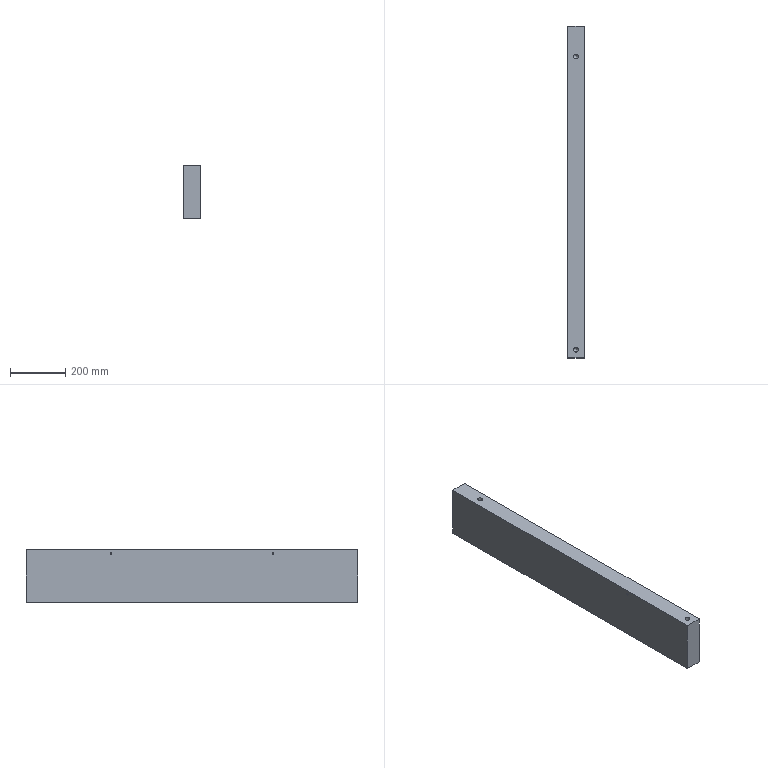Part | STEP file | lll_id4634_x_t | 1 solid | 34 faces | box 60 x 1200 x 190 mm | volume 13627617 mm3 | cylinder 14 | cone 14 | plane 6 | commonest cylinder face diameters 6.806 x10 17.506 x4
STEP:
#1=CARTESIAN_POINT('',(3946.188,490.,-370.));
#2=VERTEX_POINT('',#1);
#3=CARTESIAN_POINT('',(3937.435,490.,-370.));
#4=DIRECTION('',(0.,0.,1.));
#5=DIRECTION('',(1.,0.,0.));
#6=AXIS2_PLACEMENT_3D('',#3,#4,#5);
#7=CIRCLE('',#6,8.753);
#8=EDGE_CURVE('',#2,#2,#7,.T.);
#9=ORIENTED_EDGE('',*,*,#8,.T.);
#10=EDGE_LOOP('',(#9));
#11=FACE_BOUND('',#10,.T.);
#12=CARTESIAN_POINT('',(3907.435,-600.,-370.));
#13=VERTEX_POINT('',#12);
#14=CARTESIAN_POINT('',(3967.435,-600.,-370.));
#15=VERTEX_POINT('',#14);
#16=CARTESIAN_POINT('',(6153.751,-600.,-370.));
#17=DIRECTION('',(1.,0.,0.));
#18=VECTOR('',#17,1.);
#19=LINE('',#16,#18);
#20=EDGE_CURVE('',#13,#15,#19,.T.);
#21=ORIENTED_EDGE('',*,*,#20,.F.);
#22=CARTESIAN_POINT('',(3907.435,600.,-370.));
#23=VERTEX_POINT('',#22);
#24=CARTESIAN_POINT('',(3907.435,-1.,-370.));
#25=DIRECTION('',(0.,1.,0.));
#26=VECTOR('',#25,1.);
#27=LINE('',#24,#26);
#28=EDGE_CURVE('',#13,#23,#27,.T.);
#29=ORIENTED_EDGE('',*,*,#28,.T.);
#30=CARTESIAN_POINT('',(3967.435,600.,-370.));
#31=VERTEX_POINT('',#30);
#32=CARTESIAN_POINT('',(3967.435,600.,-370.));
#33=DIRECTION('',(-1.,0.,0.));
#34=VECTOR('',#33,1.);
#35=LINE('',#32,#34);
#36=EDGE_CURVE('',#31,#23,#35,.T.);
#37=ORIENTED_EDGE('',*,*,#36,.F.);
#38=CARTESIAN_POINT('',(3967.435,-600.,-370.));
#39=DIRECTION('',(0.,1.,0.));
#40=VECTOR('',#39,1.);
#41=LINE('',#38,#40);
#42=EDGE_CURVE('',#15,#31,#41,.T.);
#43=ORIENTED_EDGE('',*,*,#42,.F.);
#44=EDGE_LOOP('',(#21,#29,#37,#43));
#45=FACE_BOUND('',#44,.T.);
#46=CARTESIAN_POINT('',(3946.188,-490.,-370.));
#47=VERTEX_POINT('',#46);
#48=CARTESIAN_POINT('',(3937.435,-490.,-370.));
#49=DIRECTION('',(0.,0.,1.));
#50=DIRECTION('',(1.,0.,0.));
#51=AXIS2_PLACEMENT_3D('',#48,#49,#50);
#52=CIRCLE('',#51,8.753);
#53=EDGE_CURVE('',#47,#47,#52,.T.);
#54=ORIENTED_EDGE('',*,*,#53,.T.);
#55=EDGE_LOOP('',(#54));
#56=FACE_BOUND('',#55,.T.);
#57=CARTESIAN_POINT('',(6153.751,-1.,-370.));
#58=DIRECTION('',(0.,0.,-1.));
#59=DIRECTION('',(-1.,0.,0.));
#60=AXIS2_PLACEMENT_3D('',#57,#58,#59);
#61=PLANE('',#60);
#62=ADVANCED_FACE('',(#11,#45,#56),#61,.T.);
#63=CARTESIAN_POINT('',(3907.435,600.,-180.));
#64=VERTEX_POINT('',#63);
#65=CARTESIAN_POINT('',(3907.435,600.,-182.5));
#66=DIRECTION('',(0.,0.,-1.));
#67=VECTOR('',#66,1.);
#68=LINE('',#65,#67);
#69=EDGE_CURVE('',#64,#23,#68,.T.);
#70=ORIENTED_EDGE('',*,*,#69,.F.);
#71=CARTESIAN_POINT('',(3967.435,600.,-180.));
#72=VERTEX_POINT('',#71);
#73=CARTESIAN_POINT('',(6153.751,600.,-180.));
#74=DIRECTION('',(-1.,0.,0.));
#75=VECTOR('',#74,1.);
#76=LINE('',#73,#75);
#77=EDGE_CURVE('',#72,#64,#76,.T.);
#78=ORIENTED_EDGE('',*,*,#77,.F.);
#79=CARTESIAN_POINT('',(3967.435,600.,-182.5));
#80=DIRECTION('',(0.,0.,-1.));
#81=VECTOR('',#80,1.);
#82=LINE('',#79,#81);
#83=EDGE_CURVE('',#72,#31,#82,.T.);
#84=ORIENTED_EDGE('',*,*,#83,.T.);
#85=ORIENTED_EDGE('',*,*,#36,.T.);
#86=EDGE_LOOP('',(#70,#78,#84,#85));
#87=FACE_OUTER_BOUND('',#86,.T.);
#88=CARTESIAN_POINT('',(3967.435,600.,-182.5));
#89=DIRECTION('',(0.,1.,0.));
#90=DIRECTION('',(0.,0.,-1.));
#91=AXIS2_PLACEMENT_3D('',#88,#89,#90);
#92=PLANE('',#91);
#93=ADVANCED_FACE('',(#87),#92,.T.);
#94=CARTESIAN_POINT('',(3907.435,-289.597,-194.165));
#95=VERTEX_POINT('',#94);
#96=CARTESIAN_POINT('',(3907.435,-293.,-194.165));
#97=DIRECTION('',(1.,0.,0.));
#98=DIRECTION('',(0.,1.,0.));
#99=AXIS2_PLACEMENT_3D('',#96,#97,#98);
#100=CIRCLE('',#99,3.403);
#101=EDGE_CURVE('',#95,#95,#100,.T.);
#102=ORIENTED_EDGE('',*,*,#101,.T.);
#103=EDGE_LOOP('',(#102));
#104=FACE_BOUND('',#103,.T.);
#105=CARTESIAN_POINT('',(3907.435,296.403,-194.165));
#106=VERTEX_POINT('',#105);
#107=CARTESIAN_POINT('',(3907.435,293.,-194.165));
#108=DIRECTION('',(1.,0.,0.));
#109=DIRECTION('',(0.,1.,0.));
#110=AXIS2_PLACEMENT_3D('',#107,#108,#109);
#111=CIRCLE('',#110,3.403);
#112=EDGE_CURVE('',#106,#106,#111,.T.);
#113=ORIENTED_EDGE('',*,*,#112,.T.);
#114=EDGE_LOOP('',(#113));
#115=FACE_BOUND('',#114,.T.);
#116=CARTESIAN_POINT('',(3907.435,-600.,-180.));
#117=VERTEX_POINT('',#116);
#118=CARTESIAN_POINT('',(3907.435,0.,-180.));
#119=DIRECTION('',(0.,-1.,0.));
#120=VECTOR('',#119,1.);
#121=LINE('',#118,#120);
#122=EDGE_CURVE('',#64,#117,#121,.T.);
#123=ORIENTED_EDGE('',*,*,#122,.F.);
#124=ORIENTED_EDGE('',*,*,#69,.T.);
#125=ORIENTED_EDGE('',*,*,#28,.F.);
#126=CARTESIAN_POINT('',(3907.435,-600.,-160.));
#127=DIRECTION('',(0.,0.,-1.));
#128=VECTOR('',#127,1.);
#129=LINE('',#126,#128);
#130=EDGE_CURVE('',#117,#13,#129,.T.);
#131=ORIENTED_EDGE('',*,*,#130,.F.);
#132=EDGE_LOOP('',(#123,#124,#125,#131));
#133=FACE_BOUND('',#132,.T.);
#134=CARTESIAN_POINT('',(3907.435,0.,-251.25));
#135=DIRECTION('',(1.,0.,0.));
#136=DIRECTION('',(0.,0.,-1.));
#137=AXIS2_PLACEMENT_3D('',#134,#135,#136);
#138=PLANE('',#137);
#139=ADVANCED_FACE('',(#104,#115,#133),#138,.F.);
#140=CARTESIAN_POINT('',(3928.682,490.,-180.));
#141=VERTEX_POINT('',#140);
#142=CARTESIAN_POINT('',(3937.435,490.,-180.));
#143=DIRECTION('',(0.,0.,-1.));
#144=DIRECTION('',(-1.,0.,0.));
#145=AXIS2_PLACEMENT_3D('',#142,#143,#144);
#146=CIRCLE('',#145,8.753);
#147=EDGE_CURVE('',#141,#141,#146,.T.);
#148=ORIENTED_EDGE('',*,*,#147,.T.);
#149=EDGE_LOOP('',(#148));
#150=FACE_BOUND('',#149,.T.);
#151=CARTESIAN_POINT('',(3928.682,-570.,-180.));
#152=VERTEX_POINT('',#151);
#153=CARTESIAN_POINT('',(3937.435,-570.,-180.));
#154=DIRECTION('',(0.,0.,-1.));
#155=DIRECTION('',(-1.,0.,0.));
#156=AXIS2_PLACEMENT_3D('',#153,#154,#155);
#157=CIRCLE('',#156,8.753);
#158=EDGE_CURVE('',#152,#152,#157,.T.);
#159=ORIENTED_EDGE('',*,*,#158,.T.);
#160=EDGE_LOOP('',(#159));
#161=FACE_BOUND('',#160,.T.);
#162=CARTESIAN_POINT('',(3967.435,-600.,-180.));
#163=VERTEX_POINT('',#162);
#164=CARTESIAN_POINT('',(3967.435,-1.,-180.));
#165=DIRECTION('',(0.,1.,0.));
#166=VECTOR('',#165,1.);
#167=LINE('',#164,#166);
#168=EDGE_CURVE('',#163,#72,#167,.T.);
#169=ORIENTED_EDGE('',*,*,#168,.T.);
#170=ORIENTED_EDGE('',*,*,#77,.T.);
#171=ORIENTED_EDGE('',*,*,#122,.T.);
#172=CARTESIAN_POINT('',(2132.435,-600.,-180.));
#173=DIRECTION('',(-1.,0.,0.));
#174=VECTOR('',#173,1.);
#175=LINE('',#172,#174);
#176=EDGE_CURVE('',#163,#117,#175,.T.);
#177=ORIENTED_EDGE('',*,*,#176,.F.);
#178=EDGE_LOOP('',(#169,#170,#171,#177));
#179=FACE_BOUND('',#178,.T.);
#180=CARTESIAN_POINT('',(6153.751,-1.,-180.));
#181=DIRECTION('',(0.,0.,-1.));
#182=DIRECTION('',(-1.,0.,0.));
#183=AXIS2_PLACEMENT_3D('',#180,#181,#182);
#184=PLANE('',#183);
#185=ADVANCED_FACE('',(#150,#161,#179),#184,.F.);
#186=CARTESIAN_POINT('',(3967.435,402.5,-254.597));
#187=VERTEX_POINT('',#186);
#188=CARTESIAN_POINT('',(3967.435,402.5,-258.));
#189=DIRECTION('',(-1.,0.,0.));
#190=DIRECTION('',(0.,0.,1.));
#191=AXIS2_PLACEMENT_3D('',#188,#189,#190);
#192=CIRCLE('',#191,3.403);
#193=EDGE_CURVE('',#187,#187,#192,.T.);
#194=ORIENTED_EDGE('',*,*,#193,.T.);
#195=EDGE_LOOP('',(#194));
#196=FACE_BOUND('',#195,.T.);
#197=CARTESIAN_POINT('',(3967.435,412.5,-224.597));
#198=VERTEX_POINT('',#197);
#199=CARTESIAN_POINT('',(3967.435,412.5,-228.));
#200=DIRECTION('',(-1.,0.,0.));
#201=DIRECTION('',(0.,0.,1.));
#202=AXIS2_PLACEMENT_3D('',#199,#200,#201);
#203=CIRCLE('',#202,3.403);
#204=EDGE_CURVE('',#198,#198,#203,.T.);
#205=ORIENTED_EDGE('',*,*,#204,.T.);
#206=EDGE_LOOP('',(#205));
#207=FACE_BOUND('',#206,.T.);
#208=CARTESIAN_POINT('',(3967.435,62.5,-254.597));
#209=VERTEX_POINT('',#208);
#210=CARTESIAN_POINT('',(3967.435,62.5,-258.));
#211=DIRECTION('',(-1.,0.,0.));
#212=DIRECTION('',(0.,0.,1.));
#213=AXIS2_PLACEMENT_3D('',#210,#211,#212);
#214=CIRCLE('',#213,3.403);
#215=EDGE_CURVE('',#209,#209,#214,.T.);
#216=ORIENTED_EDGE('',*,*,#215,.T.);
#217=EDGE_LOOP('',(#216));
#218=FACE_BOUND('',#217,.T.);
#219=CARTESIAN_POINT('',(3967.435,72.5,-224.597));
#220=VERTEX_POINT('',#219);
#221=CARTESIAN_POINT('',(3967.435,72.5,-228.));
#222=DIRECTION('',(-1.,0.,0.));
#223=DIRECTION('',(0.,0.,1.));
#224=AXIS2_PLACEMENT_3D('',#221,#222,#223);
#225=CIRCLE('',#224,3.403);
#226=EDGE_CURVE('',#220,#220,#225,.T.);
#227=ORIENTED_EDGE('',*,*,#226,.T.);
#228=EDGE_LOOP('',(#227));
#229=FACE_BOUND('',#228,.T.);
#230=CARTESIAN_POINT('',(3967.435,-82.,-254.597));
#231=VERTEX_POINT('',#230);
#232=CARTESIAN_POINT('',(3967.435,-82.,-258.));
#233=DIRECTION('',(-1.,0.,0.));
#234=DIRECTION('',(0.,0.,1.));
#235=AXIS2_PLACEMENT_3D('',#232,#233,#234);
#236=CIRCLE('',#235,3.403);
#237=EDGE_CURVE('',#231,#231,#236,.T.);
#238=ORIENTED_EDGE('',*,*,#237,.T.);
#239=EDGE_LOOP('',(#238));
#240=FACE_BOUND('',#239,.T.);
#241=CARTESIAN_POINT('',(3967.435,-72.,-224.597));
#242=VERTEX_POINT('',#241);
#243=CARTESIAN_POINT('',(3967.435,-72.,-228.));
#244=DIRECTION('',(-1.,0.,0.));
#245=DIRECTION('',(0.,0.,1.));
#246=AXIS2_PLACEMENT_3D('',#243,#244,#245);
#247=CIRCLE('',#246,3.403);
#248=EDGE_CURVE('',#242,#242,#247,.T.);
#249=ORIENTED_EDGE('',*,*,#248,.T.);
#250=EDGE_LOOP('',(#249));
#251=FACE_BOUND('',#250,.T.);
#252=CARTESIAN_POINT('',(3967.435,-422.,-254.597));
#253=VERTEX_POINT('',#252);
#254=CARTESIAN_POINT('',(3967.435,-422.,-258.));
#255=DIRECTION('',(-1.,0.,0.));
#256=DIRECTION('',(0.,0.,1.));
#257=AXIS2_PLACEMENT_3D('',#254,#255,#256);
#258=CIRCLE('',#257,3.403);
#259=EDGE_CURVE('',#253,#253,#258,.T.);
#260=ORIENTED_EDGE('',*,*,#259,.T.);
#261=EDGE_LOOP('',(#260));
#262=FACE_BOUND('',#261,.T.);
#263=CARTESIAN_POINT('',(3967.435,-412.,-224.597));
#264=VERTEX_POINT('',#263);
#265=CARTESIAN_POINT('',(3967.435,-412.,-228.));
#266=DIRECTION('',(-1.,0.,0.));
#267=DIRECTION('',(0.,0.,1.));
#268=AXIS2_PLACEMENT_3D('',#265,#266,#267);
#269=CIRCLE('',#268,3.403);
#270=EDGE_CURVE('',#264,#264,#269,.T.);
#271=ORIENTED_EDGE('',*,*,#270,.T.);
#272=EDGE_LOOP('',(#271));
#273=FACE_BOUND('',#272,.T.);
#274=CARTESIAN_POINT('',(3967.435,-600.,-160.));
#275=DIRECTION('',(0.,0.,-1.));
#276=VECTOR('',#275,1.);
#277=LINE('',#274,#276);
#278=EDGE_CURVE('',#163,#15,#277,.T.);
#279=ORIENTED_EDGE('',*,*,#278,.T.);
#280=ORIENTED_EDGE('',*,*,#42,.T.);
#281=ORIENTED_EDGE('',*,*,#83,.F.);
#282=ORIENTED_EDGE('',*,*,#168,.F.);
#283=EDGE_LOOP('',(#279,#280,#281,#282));
#284=FACE_BOUND('',#283,.T.);
#285=CARTESIAN_POINT('',(3967.435,-600.,-182.5));
#286=DIRECTION('',(1.,0.,0.));
#287=DIRECTION('',(0.,0.,-1.));
#288=AXIS2_PLACEMENT_3D('',#285,#286,#287);
#289=PLANE('',#288);
#290=ADVANCED_FACE('',(#196,#207,#218,#229,#240,#251,#262,#273,#284),#289,.T.);
#291=ORIENTED_EDGE('',*,*,#278,.F.);
#292=ORIENTED_EDGE('',*,*,#176,.T.);
#293=ORIENTED_EDGE('',*,*,#130,.T.);
#294=ORIENTED_EDGE('',*,*,#20,.T.);
#295=EDGE_LOOP('',(#291,#292,#293,#294));
#296=FACE_OUTER_BOUND('',#295,.T.);
#297=CARTESIAN_POINT('',(2132.435,-600.,-160.));
#298=DIRECTION('',(0.,-1.,0.));
#299=DIRECTION('',(0.,0.,-1.));
#300=AXIS2_PLACEMENT_3D('',#297,#298,#299);
#301=PLANE('',#300);
#302=ADVANCED_FACE('',(#296),#301,.T.);
#303=CARTESIAN_POINT('',(3928.682,-570.,-221.253));
#304=VERTEX_POINT('',#303);
#305=CARTESIAN_POINT('',(3937.435,-570.,-221.253));
#306=DIRECTION('',(0.,0.,-1.));
#307=DIRECTION('',(-1.,0.,0.));
#308=AXIS2_PLACEMENT_3D('',#305,#306,#307);
#309=CIRCLE('',#308,8.753);
#310=EDGE_CURVE('',#304,#304,#309,.T.);
#311=ORIENTED_EDGE('',*,*,#310,.T.);
#312=EDGE_LOOP('',(#311));
#313=FACE_BOUND('',#312,.T.);
#314=ORIENTED_EDGE('',*,*,#158,.F.);
#315=EDGE_LOOP('',(#314));
#316=FACE_BOUND('',#315,.T.);
#317=CARTESIAN_POINT('',(3937.435,-570.,-180.));
#318=DIRECTION('',(0.,0.,-1.));
#319=DIRECTION('',(1.,0.,0.));
#320=AXIS2_PLACEMENT_3D('',#317,#318,#319);
#321=CYLINDRICAL_SURFACE('',#320,8.753);
#322=ADVANCED_FACE('',(#313,#316),#321,.F.);
#323=CARTESIAN_POINT('',(3937.435,-570.,-230.006));
#324=VERTEX_POINT('',#323);
#325=VERTEX_LOOP('',#324);
#326=FACE_BOUND('',#325,.T.);
#327=ORIENTED_EDGE('',*,*,#310,.F.);
#328=EDGE_LOOP('',(#327));
#329=FACE_BOUND('',#328,.T.);
#330=CARTESIAN_POINT('',(3937.435,-570.,-221.253));
#331=DIRECTION('',(0.,0.,1.));
#332=DIRECTION('',(-1.,0.,0.));
#333=AXIS2_PLACEMENT_3D('',#330,#331,#332);
#334=CONICAL_SURFACE('',#333,8.753,45.);
#335=ADVANCED_FACE('',(#326,#329),#334,.F.);
#336=CARTESIAN_POINT('',(3928.682,490.,-221.253));
#337=VERTEX_POINT('',#336);
#338=CARTESIAN_POINT('',(3937.435,490.,-221.253));
#339=DIRECTION('',(0.,0.,-1.));
#340=DIRECTION('',(-1.,0.,0.));
#341=AXIS2_PLACEMENT_3D('',#338,#339,#340);
#342=CIRCLE('',#341,8.753);
#343=EDGE_CURVE('',#337,#337,#342,.T.);
#344=ORIENTED_EDGE('',*,*,#343,.T.);
#345=EDGE_LOOP('',(#344));
#346=FACE_BOUND('',#345,.T.);
#347=ORIENTED_EDGE('',*,*,#147,.F.);
#348=EDGE_LOOP('',(#347));
#349=FACE_BOUND('',#348,.T.);
#350=CARTESIAN_POINT('',(3937.435,490.,-180.));
#351=DIRECTION('',(0.,0.,-1.));
#352=DIRECTION('',(1.,0.,0.));
#353=AXIS2_PLACEMENT_3D('',#350,#351,#352);
#354=CYLINDRICAL_SURFACE('',#353,8.753);
#355=ADVANCED_FACE('',(#346,#349),#354,.F.);
#356=CARTESIAN_POINT('',(3937.435,490.,-230.006));
#357=VERTEX_POINT('',#356);
#358=VERTEX_LOOP('',#357);
#359=FACE_BOUND('',#358,.T.);
#360=ORIENTED_EDGE('',*,*,#343,.F.);
#361=EDGE_LOOP('',(#360));
#362=FACE_BOUND('',#361,.T.);
#363=CARTESIAN_POINT('',(3937.435,490.,-221.253));
#364=DIRECTION('',(0.,0.,1.));
#365=DIRECTION('',(-1.,0.,0.));
#366=AXIS2_PLACEMENT_3D('',#363,#364,#365);
#367=CONICAL_SURFACE('',#366,8.753,45.);
#368=ADVANCED_FACE('',(#359,#362),#367,.F.);
#369=CARTESIAN_POINT('',(3946.188,490.,-328.747));
#370=VERTEX_POINT('',#369);
#371=CARTESIAN_POINT('',(3937.435,490.,-328.747));
#372=DIRECTION('',(0.,0.,1.));
#373=DIRECTION('',(1.,0.,0.));
#374=AXIS2_PLACEMENT_3D('',#371,#372,#373);
#375=CIRCLE('',#374,8.753);
#376=EDGE_CURVE('',#370,#370,#375,.T.);
#377=ORIENTED_EDGE('',*,*,#376,.T.);
#378=EDGE_LOOP('',(#377));
#379=FACE_BOUND('',#378,.T.);
#380=ORIENTED_EDGE('',*,*,#8,.F.);
#381=EDGE_LOOP('',(#380));
#382=FACE_BOUND('',#381,.T.);
#383=CARTESIAN_POINT('',(3937.435,490.,-370.));
#384=DIRECTION('',(0.,0.,1.));
#385=DIRECTION('',(-1.,0.,0.));
#386=AXIS2_PLACEMENT_3D('',#383,#384,#385);
#387=CYLINDRICAL_SURFACE('',#386,8.753);
#388=ADVANCED_FACE('',(#379,#382),#387,.F.);
#389=CARTESIAN_POINT('',(3937.435,490.,-319.994));
#390=VERTEX_POINT('',#389);
#391=VERTEX_LOOP('',#390);
#392=FACE_BOUND('',#391,.T.);
#393=ORIENTED_EDGE('',*,*,#376,.F.);
#394=EDGE_LOOP('',(#393));
#395=FACE_BOUND('',#394,.T.);
#396=CARTESIAN_POINT('',(3937.435,490.,-328.747));
#397=DIRECTION('',(0.,0.,-1.));
#398=DIRECTION('',(1.,0.,0.));
#399=AXIS2_PLACEMENT_3D('',#396,#397,#398);
#400=CONICAL_SURFACE('',#399,8.753,45.);
#401=ADVANCED_FACE('',(#392,#395),#400,.F.);
#402=CARTESIAN_POINT('',(3946.188,-490.,-328.747));
#403=VERTEX_POINT('',#402);
#404=CARTESIAN_POINT('',(3937.435,-490.,-328.747));
#405=DIRECTION('',(0.,0.,1.));
#406=DIRECTION('',(1.,0.,0.));
#407=AXIS2_PLACEMENT_3D('',#404,#405,#406);
#408=CIRCLE('',#407,8.753);
#409=EDGE_CURVE('',#403,#403,#408,.T.);
#410=ORIENTED_EDGE('',*,*,#409,.T.);
#411=EDGE_LOOP('',(#410));
#412=FACE_BOUND('',#411,.T.);
#413=ORIENTED_EDGE('',*,*,#53,.F.);
#414=EDGE_LOOP('',(#413));
#415=FACE_BOUND('',#414,.T.);
#416=CARTESIAN_POINT('',(3937.435,-490.,-370.));
#417=DIRECTION('',(0.,0.,1.));
#418=DIRECTION('',(-1.,0.,0.));
#419=AXIS2_PLACEMENT_3D('',#416,#417,#418);
#420=CYLINDRICAL_SURFACE('',#419,8.753);
#421=ADVANCED_FACE('',(#412,#415),#420,.F.);
#422=CARTESIAN_POINT('',(3937.435,-490.,-319.994));
#423=VERTEX_POINT('',#422);
#424=VERTEX_LOOP('',#423);
#425=FACE_BOUND('',#424,.T.);
#426=ORIENTED_EDGE('',*,*,#409,.F.);
#427=EDGE_LOOP('',(#426));
#428=FACE_BOUND('',#427,.T.);
#429=CARTESIAN_POINT('',(3937.435,-490.,-328.747));
#430=DIRECTION('',(0.,0.,-1.));
#431=DIRECTION('',(1.,0.,0.));
#432=AXIS2_PLACEMENT_3D('',#429,#430,#431);
#433=CONICAL_SURFACE('',#432,8.753,45.);
#434=ADVANCED_FACE('',(#425,#428),#433,.F.);
#435=CARTESIAN_POINT('',(3942.435,-412.,-224.597));
#436=VERTEX_POINT('',#435);
#437=CARTESIAN_POINT('',(3942.435,-412.,-228.));
#438=DIRECTION('',(1.,0.,0.));
#439=DIRECTION('',(0.,0.,1.));
#440=AXIS2_PLACEMENT_3D('',#437,#438,#439);
#441=CIRCLE('',#440,3.403);
#442=EDGE_CURVE('',#436,#436,#441,.T.);
#443=ORIENTED_EDGE('',*,*,#442,.T.);
#444=EDGE_LOOP('',(#443));
#445=FACE_BOUND('',#444,.T.);
#446=CARTESIAN_POINT('',(3940.391,-412.,-228.));
#447=VERTEX_POINT('',#446);
#448=VERTEX_LOOP('',#447);
#449=FACE_BOUND('',#448,.T.);
#450=CARTESIAN_POINT('',(3942.435,-412.,-228.));
#451=DIRECTION('',(1.,0.,0.));
#452=DIRECTION('',(0.,0.,1.));
#453=AXIS2_PLACEMENT_3D('',#450,#451,#452);
#454=CONICAL_SURFACE('',#453,3.403,59.);
#455=ADVANCED_FACE('',(#445,#449),#454,.F.);
#456=ORIENTED_EDGE('',*,*,#442,.F.);
#457=EDGE_LOOP('',(#456));
#458=FACE_BOUND('',#457,.T.);
#459=ORIENTED_EDGE('',*,*,#270,.F.);
#460=EDGE_LOOP('',(#459));
#461=FACE_BOUND('',#460,.T.);
#462=CARTESIAN_POINT('',(3967.435,-412.,-228.));
#463=DIRECTION('',(-1.,0.,0.));
#464=DIRECTION('',(0.,0.,-1.));
#465=AXIS2_PLACEMENT_3D('',#462,#463,#464);
#466=CYLINDRICAL_SURFACE('',#465,3.403);
#467=ADVANCED_FACE('',(#458,#461),#466,.F.);
#468=CARTESIAN_POINT('',(3942.435,-422.,-254.597));
#469=VERTEX_POINT('',#468);
#470=CARTESIAN_POINT('',(3942.435,-422.,-258.));
#471=DIRECTION('',(1.,0.,0.));
#472=DIRECTION('',(0.,0.,1.));
#473=AXIS2_PLACEMENT_3D('',#470,#471,#472);
#474=CIRCLE('',#473,3.403);
#475=EDGE_CURVE('',#469,#469,#474,.T.);
#476=ORIENTED_EDGE('',*,*,#475,.T.);
#477=EDGE_LOOP('',(#476));
#478=FACE_BOUND('',#477,.T.);
#479=CARTESIAN_POINT('',(3940.391,-422.,-258.));
#480=VERTEX_POINT('',#479);
#481=VERTEX_LOOP('',#480);
#482=FACE_BOUND('',#481,.T.);
#483=CARTESIAN_POINT('',(3942.435,-422.,-258.));
#484=DIRECTION('',(1.,0.,0.));
#485=DIRECTION('',(0.,0.,1.));
#486=AXIS2_PLACEMENT_3D('',#483,#484,#485);
#487=CONICAL_SURFACE('',#486,3.403,59.);
#488=ADVANCED_FACE('',(#478,#482),#487,.F.);
#489=ORIENTED_EDGE('',*,*,#475,.F.);
#490=EDGE_LOOP('',(#489));
#491=FACE_BOUND('',#490,.T.);
#492=ORIENTED_EDGE('',*,*,#259,.F.);
#493=EDGE_LOOP('',(#492));
#494=FACE_BOUND('',#493,.T.);
#495=CARTESIAN_POINT('',(3967.435,-422.,-258.));
#496=DIRECTION('',(-1.,0.,0.));
#497=DIRECTION('',(0.,0.,-1.));
#498=AXIS2_PLACEMENT_3D('',#495,#496,#497);
#499=CYLINDRICAL_SURFACE('',#498,3.403);
#500=ADVANCED_FACE('',(#491,#494),#499,.F.);
#501=CARTESIAN_POINT('',(3942.435,-72.,-224.597));
#502=VERTEX_POINT('',#501);
#503=CARTESIAN_POINT('',(3942.435,-72.,-228.));
#504=DIRECTION('',(1.,0.,0.));
#505=DIRECTION('',(0.,0.,1.));
#506=AXIS2_PLACEMENT_3D('',#503,#504,#505);
#507=CIRCLE('',#506,3.403);
#508=EDGE_CURVE('',#502,#502,#507,.T.);
#509=ORIENTED_EDGE('',*,*,#508,.T.);
#510=EDGE_LOOP('',(#509));
#511=FACE_BOUND('',#510,.T.);
#512=CARTESIAN_POINT('',(3940.391,-72.,-228.));
#513=VERTEX_POINT('',#512);
#514=VERTEX_LOOP('',#513);
#515=FACE_BOUND('',#514,.T.);
#516=CARTESIAN_POINT('',(3942.435,-72.,-228.));
#517=DIRECTION('',(1.,0.,0.));
#518=DIRECTION('',(0.,0.,1.));
#519=AXIS2_PLACEMENT_3D('',#516,#517,#518);
#520=CONICAL_SURFACE('',#519,3.403,59.);
#521=ADVANCED_FACE('',(#511,#515),#520,.F.);
#522=ORIENTED_EDGE('',*,*,#508,.F.);
#523=EDGE_LOOP('',(#522));
#524=FACE_BOUND('',#523,.T.);
#525=ORIENTED_EDGE('',*,*,#248,.F.);
#526=EDGE_LOOP('',(#525));
#527=FACE_BOUND('',#526,.T.);
#528=CARTESIAN_POINT('',(3967.435,-72.,-228.));
#529=DIRECTION('',(-1.,0.,0.));
#530=DIRECTION('',(0.,0.,-1.));
#531=AXIS2_PLACEMENT_3D('',#528,#529,#530);
#532=CYLINDRICAL_SURFACE('',#531,3.403);
#533=ADVANCED_FACE('',(#524,#527),#532,.F.);
#534=CARTESIAN_POINT('',(3942.435,-82.,-254.597));
#535=VERTEX_POINT('',#534);
#536=CARTESIAN_POINT('',(3942.435,-82.,-258.));
#537=DIRECTION('',(1.,0.,0.));
#538=DIRECTION('',(0.,0.,1.));
#539=AXIS2_PLACEMENT_3D('',#536,#537,#538);
#540=CIRCLE('',#539,3.403);
#541=EDGE_CURVE('',#535,#535,#540,.T.);
#542=ORIENTED_EDGE('',*,*,#541,.T.);
#543=EDGE_LOOP('',(#542));
#544=FACE_BOUND('',#543,.T.);
#545=CARTESIAN_POINT('',(3940.391,-82.,-258.));
#546=VERTEX_POINT('',#545);
#547=VERTEX_LOOP('',#546);
#548=FACE_BOUND('',#547,.T.);
#549=CARTESIAN_POINT('',(3942.435,-82.,-258.));
#550=DIRECTION('',(1.,0.,0.));
#551=DIRECTION('',(0.,0.,1.));
#552=AXIS2_PLACEMENT_3D('',#549,#550,#551);
#553=CONICAL_SURFACE('',#552,3.403,59.);
#554=ADVANCED_FACE('',(#544,#548),#553,.F.);
#555=ORIENTED_EDGE('',*,*,#541,.F.);
#556=EDGE_LOOP('',(#555));
#557=FACE_BOUND('',#556,.T.);
#558=ORIENTED_EDGE('',*,*,#237,.F.);
#559=EDGE_LOOP('',(#558));
#560=FACE_BOUND('',#559,.T.);
#561=CARTESIAN_POINT('',(3967.435,-82.,-258.));
#562=DIRECTION('',(-1.,0.,0.));
#563=DIRECTION('',(0.,0.,-1.));
#564=AXIS2_PLACEMENT_3D('',#561,#562,#563);
#565=CYLINDRICAL_SURFACE('',#564,3.403);
#566=ADVANCED_FACE('',(#557,#560),#565,.F.);
#567=CARTESIAN_POINT('',(3942.435,72.5,-224.597));
#568=VERTEX_POINT('',#567);
#569=CARTESIAN_POINT('',(3942.435,72.5,-228.));
#570=DIRECTION('',(1.,0.,0.));
#571=DIRECTION('',(0.,0.,1.));
#572=AXIS2_PLACEMENT_3D('',#569,#570,#571);
#573=CIRCLE('',#572,3.403);
#574=EDGE_CURVE('',#568,#568,#573,.T.);
#575=ORIENTED_EDGE('',*,*,#574,.T.);
#576=EDGE_LOOP('',(#575));
#577=FACE_BOUND('',#576,.T.);
#578=CARTESIAN_POINT('',(3940.391,72.5,-228.));
#579=VERTEX_POINT('',#578);
#580=VERTEX_LOOP('',#579);
#581=FACE_BOUND('',#580,.T.);
#582=CARTESIAN_POINT('',(3942.435,72.5,-228.));
#583=DIRECTION('',(1.,0.,0.));
#584=DIRECTION('',(0.,0.,1.));
#585=AXIS2_PLACEMENT_3D('',#582,#583,#584);
#586=CONICAL_SURFACE('',#585,3.403,59.);
#587=ADVANCED_FACE('',(#577,#581),#586,.F.);
#588=ORIENTED_EDGE('',*,*,#574,.F.);
#589=EDGE_LOOP('',(#588));
#590=FACE_BOUND('',#589,.T.);
#591=ORIENTED_EDGE('',*,*,#226,.F.);
#592=EDGE_LOOP('',(#591));
#593=FACE_BOUND('',#592,.T.);
#594=CARTESIAN_POINT('',(3967.435,72.5,-228.));
#595=DIRECTION('',(-1.,0.,0.));
#596=DIRECTION('',(0.,0.,-1.));
#597=AXIS2_PLACEMENT_3D('',#594,#595,#596);
#598=CYLINDRICAL_SURFACE('',#597,3.403);
#599=ADVANCED_FACE('',(#590,#593),#598,.F.);
#600=CARTESIAN_POINT('',(3942.435,62.5,-254.597));
#601=VERTEX_POINT('',#600);
#602=CARTESIAN_POINT('',(3942.435,62.5,-258.));
#603=DIRECTION('',(1.,0.,0.));
#604=DIRECTION('',(0.,0.,1.));
#605=AXIS2_PLACEMENT_3D('',#602,#603,#604);
#606=CIRCLE('',#605,3.403);
#607=EDGE_CURVE('',#601,#601,#606,.T.);
#608=ORIENTED_EDGE('',*,*,#607,.T.);
#609=EDGE_LOOP('',(#608));
#610=FACE_BOUND('',#609,.T.);
#611=CARTESIAN_POINT('',(3940.391,62.5,-258.));
#612=VERTEX_POINT('',#611);
#613=VERTEX_LOOP('',#612);
#614=FACE_BOUND('',#613,.T.);
#615=CARTESIAN_POINT('',(3942.435,62.5,-258.));
#616=DIRECTION('',(1.,0.,0.));
#617=DIRECTION('',(0.,0.,1.));
#618=AXIS2_PLACEMENT_3D('',#615,#616,#617);
#619=CONICAL_SURFACE('',#618,3.403,59.);
#620=ADVANCED_FACE('',(#610,#614),#619,.F.);
#621=ORIENTED_EDGE('',*,*,#607,.F.);
#622=EDGE_LOOP('',(#621));
#623=FACE_BOUND('',#622,.T.);
#624=ORIENTED_EDGE('',*,*,#215,.F.);
#625=EDGE_LOOP('',(#624));
#626=FACE_BOUND('',#625,.T.);
#627=CARTESIAN_POINT('',(3967.435,62.5,-258.));
#628=DIRECTION('',(-1.,0.,0.));
#629=DIRECTION('',(0.,0.,-1.));
#630=AXIS2_PLACEMENT_3D('',#627,#628,#629);
#631=CYLINDRICAL_SURFACE('',#630,3.403);
#632=ADVANCED_FACE('',(#623,#626),#631,.F.);
#633=CARTESIAN_POINT('',(3942.435,412.5,-224.597));
#634=VERTEX_POINT('',#633);
#635=CARTESIAN_POINT('',(3942.435,412.5,-228.));
#636=DIRECTION('',(1.,0.,0.));
#637=DIRECTION('',(0.,0.,1.));
#638=AXIS2_PLACEMENT_3D('',#635,#636,#637);
#639=CIRCLE('',#638,3.403);
#640=EDGE_CURVE('',#634,#634,#639,.T.);
#641=ORIENTED_EDGE('',*,*,#640,.T.);
#642=EDGE_LOOP('',(#641));
#643=FACE_BOUND('',#642,.T.);
#644=CARTESIAN_POINT('',(3940.391,412.5,-228.));
#645=VERTEX_POINT('',#644);
#646=VERTEX_LOOP('',#645);
#647=FACE_BOUND('',#646,.T.);
#648=CARTESIAN_POINT('',(3942.435,412.5,-228.));
#649=DIRECTION('',(1.,0.,0.));
#650=DIRECTION('',(0.,0.,1.));
#651=AXIS2_PLACEMENT_3D('',#648,#649,#650);
#652=CONICAL_SURFACE('',#651,3.403,59.);
#653=ADVANCED_FACE('',(#643,#647),#652,.F.);
#654=ORIENTED_EDGE('',*,*,#640,.F.);
#655=EDGE_LOOP('',(#654));
#656=FACE_BOUND('',#655,.T.);
#657=ORIENTED_EDGE('',*,*,#204,.F.);
#658=EDGE_LOOP('',(#657));
#659=FACE_BOUND('',#658,.T.);
#660=CARTESIAN_POINT('',(3967.435,412.5,-228.));
#661=DIRECTION('',(-1.,0.,0.));
#662=DIRECTION('',(0.,0.,-1.));
#663=AXIS2_PLACEMENT_3D('',#660,#661,#662);
#664=CYLINDRICAL_SURFACE('',#663,3.403);
#665=ADVANCED_FACE('',(#656,#659),#664,.F.);
#666=CARTESIAN_POINT('',(3942.435,402.5,-254.597));
#667=VERTEX_POINT('',#666);
#668=CARTESIAN_POINT('',(3942.435,402.5,-258.));
#669=DIRECTION('',(1.,0.,0.));
#670=DIRECTION('',(0.,0.,1.));
#671=AXIS2_PLACEMENT_3D('',#668,#669,#670);
#672=CIRCLE('',#671,3.403);
#673=EDGE_CURVE('',#667,#667,#672,.T.);
#674=ORIENTED_EDGE('',*,*,#673,.T.);
#675=EDGE_LOOP('',(#674));
#676=FACE_BOUND('',#675,.T.);
#677=CARTESIAN_POINT('',(3940.391,402.5,-258.));
#678=VERTEX_POINT('',#677);
#679=VERTEX_LOOP('',#678);
#680=FACE_BOUND('',#679,.T.);
#681=CARTESIAN_POINT('',(3942.435,402.5,-258.));
#682=DIRECTION('',(1.,0.,0.));
#683=DIRECTION('',(0.,0.,1.));
#684=AXIS2_PLACEMENT_3D('',#681,#682,#683);
#685=CONICAL_SURFACE('',#684,3.403,59.);
#686=ADVANCED_FACE('',(#676,#680),#685,.F.);
#687=ORIENTED_EDGE('',*,*,#673,.F.);
#688=EDGE_LOOP('',(#687));
#689=FACE_BOUND('',#688,.T.);
#690=ORIENTED_EDGE('',*,*,#193,.F.);
#691=EDGE_LOOP('',(#690));
#692=FACE_BOUND('',#691,.T.);
#693=CARTESIAN_POINT('',(3967.435,402.5,-258.));
#694=DIRECTION('',(-1.,0.,0.));
#695=DIRECTION('',(0.,0.,-1.));
#696=AXIS2_PLACEMENT_3D('',#693,#694,#695);
#697=CYLINDRICAL_SURFACE('',#696,3.403);
#698=ADVANCED_FACE('',(#689,#692),#697,.F.);
#699=CARTESIAN_POINT('',(3939.038,293.,-197.568));
#700=VERTEX_POINT('',#699);
#701=CARTESIAN_POINT('',(3939.038,293.,-194.165));
#702=DIRECTION('',(1.,0.,0.));
#703=DIRECTION('',(0.,0.,-1.));
#704=AXIS2_PLACEMENT_3D('',#701,#702,#703);
#705=CIRCLE('',#704,3.403);
#706=EDGE_CURVE('',#700,#700,#705,.T.);
#707=ORIENTED_EDGE('',*,*,#706,.T.);
#708=EDGE_LOOP('',(#707));
#709=FACE_BOUND('',#708,.T.);
#710=ORIENTED_EDGE('',*,*,#112,.F.);
#711=EDGE_LOOP('',(#710));
#712=FACE_BOUND('',#711,.T.);
#713=CARTESIAN_POINT('',(3907.435,293.,-194.165));
#714=DIRECTION('',(1.,0.,0.));
#715=DIRECTION('',(0.,-1.,0.));
#716=AXIS2_PLACEMENT_3D('',#713,#714,#715);
#717=CYLINDRICAL_SURFACE('',#716,3.403);
#718=ADVANCED_FACE('',(#709,#712),#717,.F.);
#719=CARTESIAN_POINT('',(3942.441,293.,-194.165));
#720=VERTEX_POINT('',#719);
#721=VERTEX_LOOP('',#720);
#722=FACE_BOUND('',#721,.T.);
#723=ORIENTED_EDGE('',*,*,#706,.F.);
#724=EDGE_LOOP('',(#723));
#725=FACE_BOUND('',#724,.T.);
#726=CARTESIAN_POINT('',(3939.038,293.,-194.165));
#727=DIRECTION('',(-1.,0.,0.));
#728=DIRECTION('',(0.,0.,-1.));
#729=AXIS2_PLACEMENT_3D('',#726,#727,#728);
#730=CONICAL_SURFACE('',#729,3.403,45.);
#731=ADVANCED_FACE('',(#722,#725),#730,.F.);
#732=CARTESIAN_POINT('',(3939.038,-293.,-197.568));
#733=VERTEX_POINT('',#732);
#734=CARTESIAN_POINT('',(3939.038,-293.,-194.165));
#735=DIRECTION('',(1.,0.,0.));
#736=DIRECTION('',(0.,0.,-1.));
#737=AXIS2_PLACEMENT_3D('',#734,#735,#736);
#738=CIRCLE('',#737,3.403);
#739=EDGE_CURVE('',#733,#733,#738,.T.);
#740=ORIENTED_EDGE('',*,*,#739,.T.);
#741=EDGE_LOOP('',(#740));
#742=FACE_BOUND('',#741,.T.);
#743=ORIENTED_EDGE('',*,*,#101,.F.);
#744=EDGE_LOOP('',(#743));
#745=FACE_BOUND('',#744,.T.);
#746=CARTESIAN_POINT('',(3907.435,-293.,-194.165));
#747=DIRECTION('',(1.,0.,0.));
#748=DIRECTION('',(0.,-1.,0.));
#749=AXIS2_PLACEMENT_3D('',#746,#747,#748);
#750=CYLINDRICAL_SURFACE('',#749,3.403);
#751=ADVANCED_FACE('',(#742,#745),#750,.F.);
#752=CARTESIAN_POINT('',(3942.441,-293.,-194.165));
#753=VERTEX_POINT('',#752);
#754=VERTEX_LOOP('',#753);
#755=FACE_BOUND('',#754,.T.);
#756=ORIENTED_EDGE('',*,*,#739,.F.);
#757=EDGE_LOOP('',(#756));
#758=FACE_BOUND('',#757,.T.);
#759=CARTESIAN_POINT('',(3939.038,-293.,-194.165));
#760=DIRECTION('',(-1.,0.,0.));
#761=DIRECTION('',(0.,0.,-1.));
#762=AXIS2_PLACEMENT_3D('',#759,#760,#761);
#763=CONICAL_SURFACE('',#762,3.403,45.);
#764=ADVANCED_FACE('',(#755,#758),#763,.F.);
#765=CLOSED_SHELL('',(#62,#93,#139,#185,#290,#302,#322,#335,#355,#368,#388,#401,#421,#434,#455,#467,#488,#500,#521,#533,#554,#566,#587,#599,#620,#632,#653,#665,#686,#698,#718,#731,#751,#764));
#766=MANIFOLD_SOLID_BREP('',#765);
#767=(LENGTH_UNIT()NAMED_UNIT(*)SI_UNIT(.MILLI.,.METRE.));
#768=UNCERTAINTY_MEASURE_WITH_UNIT(LENGTH_MEASURE(0.00002),#767,'','');
#769=(NAMED_UNIT(*)PLANE_ANGLE_UNIT()SI_UNIT($,.RADIAN.));
#770=PLANE_ANGLE_MEASURE_WITH_UNIT(PLANE_ANGLE_MEASURE(0.01745),#769);
#771=DIMENSIONAL_EXPONENTS(0.,0.,0.,0.,0.,0.,0.);
#772=(CONVERSION_BASED_UNIT('DEGREE',#770)NAMED_UNIT(#771)PLANE_ANGLE_UNIT());
#773=(NAMED_UNIT(*)SI_UNIT($,.STERADIAN.)SOLID_ANGLE_UNIT());
#774=(GEOMETRIC_REPRESENTATION_CONTEXT(3)GLOBAL_UNCERTAINTY_ASSIGNED_CONTEXT((#768))GLOBAL_UNIT_ASSIGNED_CONTEXT((#767,#772,#773))REPRESENTATION_CONTEXT('',''));
#775=ADVANCED_BREP_SHAPE_REPRESENTATION('',(#766),#774);